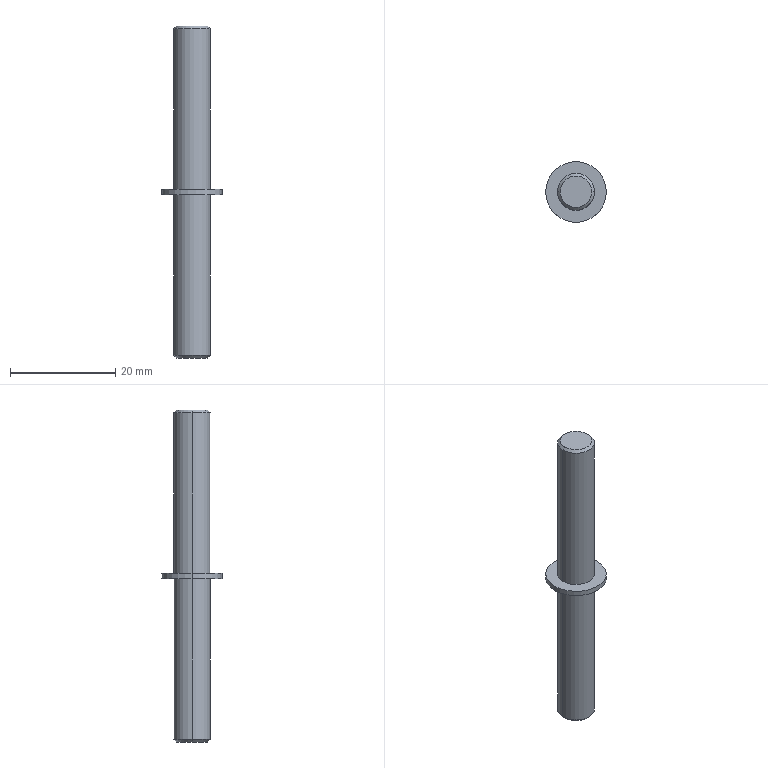Part | NX | features BREP 1 | 1 solid | 14 faces | box 11.5 x 11.5 x 63 mm | volume 2485 mm3 | cylinder 6 | cone 4 | plane 4 | commonest cylinder face diameters 7 x4 11.5 x2
STEP:
#1=CARTESIAN_POINT('',(-3.5,0.,31.));
#2=VERTEX_POINT('',#1);
#3=CARTESIAN_POINT('',(3.5,0.,31.));
#4=VERTEX_POINT('',#3);
#5=CARTESIAN_POINT('',(0.,0.,31.));
#6=DIRECTION('',(0.,0.,-1.));
#7=DIRECTION('',(1.,0.,0.));
#8=AXIS2_PLACEMENT_3D('',#5,#6,#7);
#9=CIRCLE('',#8,3.5);
#10=EDGE_CURVE('',#2,#4,#9,.T.);
#11=ORIENTED_EDGE('',*,*,#10,.T.);
#12=CARTESIAN_POINT('',(3.5,0.,0.5));
#13=VERTEX_POINT('',#12);
#14=CARTESIAN_POINT('',(3.5,0.,31.5));
#15=DIRECTION('',(0.,0.,-1.));
#16=VECTOR('',#15,1000.);
#17=LINE('',#14,#16);
#18=EDGE_CURVE('',#4,#13,#17,.T.);
#19=ORIENTED_EDGE('',*,*,#18,.T.);
#20=CARTESIAN_POINT('',(-3.5,0.,0.5));
#21=VERTEX_POINT('',#20);
#22=CARTESIAN_POINT('',(0.,0.,0.5));
#23=DIRECTION('',(0.,0.,-1.));
#24=DIRECTION('',(-1.,0.,0.));
#25=AXIS2_PLACEMENT_3D('',#22,#23,#24);
#26=CIRCLE('',#25,3.5);
#27=EDGE_CURVE('',#21,#13,#26,.T.);
#28=ORIENTED_EDGE('',*,*,#27,.F.);
#29=CARTESIAN_POINT('',(-3.5,0.,31.5));
#30=DIRECTION('',(0.,0.,-1.));
#31=VECTOR('',#30,1000.);
#32=LINE('',#29,#31);
#33=EDGE_CURVE('',#2,#21,#32,.T.);
#34=ORIENTED_EDGE('',*,*,#33,.F.);
#35=EDGE_LOOP('',(#11,#19,#28,#34));
#36=FACE_BOUND('',#35,.T.);
#37=CARTESIAN_POINT('',(0.,0.,31.5));
#38=DIRECTION('',(0.,0.,-1.));
#39=DIRECTION('',(-1.,0.,0.));
#40=AXIS2_PLACEMENT_3D('',#37,#38,#39);
#41=CYLINDRICAL_SURFACE('',#40,3.5);
#42=ADVANCED_FACE('',(#36),#41,.T.);
#43=CARTESIAN_POINT('',(3.,0.,31.5));
#44=VERTEX_POINT('',#43);
#45=CARTESIAN_POINT('',(-3.,0.,31.5));
#46=VERTEX_POINT('',#45);
#47=CARTESIAN_POINT('',(0.,0.,31.5));
#48=DIRECTION('',(0.,0.,1.));
#49=DIRECTION('',(1.,0.,0.));
#50=AXIS2_PLACEMENT_3D('',#47,#48,#49);
#51=CIRCLE('',#50,3.);
#52=EDGE_CURVE('',#44,#46,#51,.T.);
#53=ORIENTED_EDGE('',*,*,#52,.F.);
#54=CARTESIAN_POINT('',(3.,0.,31.5));
#55=DIRECTION('',(0.7071,0.,-0.7071));
#56=VECTOR('',#55,1000.);
#57=LINE('',#54,#56);
#58=EDGE_CURVE('',#44,#4,#57,.T.);
#59=ORIENTED_EDGE('',*,*,#58,.T.);
#60=ORIENTED_EDGE('',*,*,#10,.F.);
#61=CARTESIAN_POINT('',(-3.,0.,31.5));
#62=DIRECTION('',(-0.7071,0.,-0.7071));
#63=VECTOR('',#62,1000.);
#64=LINE('',#61,#63);
#65=EDGE_CURVE('',#46,#2,#64,.T.);
#66=ORIENTED_EDGE('',*,*,#65,.F.);
#67=EDGE_LOOP('',(#53,#59,#60,#66));
#68=FACE_BOUND('',#67,.T.);
#69=CARTESIAN_POINT('',(0.,0.,31.5));
#70=DIRECTION('',(0.,0.,-1.));
#71=DIRECTION('',(-1.,0.,0.));
#72=AXIS2_PLACEMENT_3D('',#69,#70,#71);
#73=CONICAL_SURFACE('',#72,3.,0.7854);
#74=ADVANCED_FACE('',(#68),#73,.T.);
#75=CARTESIAN_POINT('',(-5.75,0.,0.5));
#76=VERTEX_POINT('',#75);
#77=CARTESIAN_POINT('',(5.75,0.,0.5));
#78=VERTEX_POINT('',#77);
#79=CARTESIAN_POINT('',(0.,0.,0.5));
#80=DIRECTION('',(0.,0.,-1.));
#81=DIRECTION('',(-1.,0.,0.));
#82=AXIS2_PLACEMENT_3D('',#79,#80,#81);
#83=CIRCLE('',#82,5.75);
#84=EDGE_CURVE('',#76,#78,#83,.T.);
#85=ORIENTED_EDGE('',*,*,#84,.T.);
#86=CARTESIAN_POINT('',(5.75,0.,-0.5));
#87=VERTEX_POINT('',#86);
#88=CARTESIAN_POINT('',(5.75,0.,0.));
#89=DIRECTION('',(0.,0.,-1.));
#90=VECTOR('',#89,1000.);
#91=LINE('',#88,#90);
#92=EDGE_CURVE('',#78,#87,#91,.T.);
#93=ORIENTED_EDGE('',*,*,#92,.T.);
#94=CARTESIAN_POINT('',(-5.75,0.,-0.5));
#95=VERTEX_POINT('',#94);
#96=CARTESIAN_POINT('',(0.,0.,-0.5));
#97=DIRECTION('',(0.,0.,-1.));
#98=DIRECTION('',(-1.,0.,0.));
#99=AXIS2_PLACEMENT_3D('',#96,#97,#98);
#100=CIRCLE('',#99,5.75);
#101=EDGE_CURVE('',#95,#87,#100,.T.);
#102=ORIENTED_EDGE('',*,*,#101,.F.);
#103=CARTESIAN_POINT('',(-5.75,0.,0.));
#104=DIRECTION('',(0.,0.,-1.));
#105=VECTOR('',#104,1000.);
#106=LINE('',#103,#105);
#107=EDGE_CURVE('',#76,#95,#106,.T.);
#108=ORIENTED_EDGE('',*,*,#107,.F.);
#109=EDGE_LOOP('',(#85,#93,#102,#108));
#110=FACE_BOUND('',#109,.T.);
#111=CARTESIAN_POINT('',(0.,0.,0.));
#112=DIRECTION('',(0.,0.,-1.));
#113=DIRECTION('',(-1.,0.,0.));
#114=AXIS2_PLACEMENT_3D('',#111,#112,#113);
#115=CYLINDRICAL_SURFACE('',#114,5.75);
#116=ADVANCED_FACE('',(#110),#115,.T.);
#117=CARTESIAN_POINT('',(-3.,0.,-31.5));
#118=VERTEX_POINT('',#117);
#119=CARTESIAN_POINT('',(3.,0.,-31.5));
#120=VERTEX_POINT('',#119);
#121=CARTESIAN_POINT('',(0.,0.,-31.5));
#122=DIRECTION('',(0.,0.,-1.));
#123=DIRECTION('',(1.,0.,0.));
#124=AXIS2_PLACEMENT_3D('',#121,#122,#123);
#125=CIRCLE('',#124,3.);
#126=EDGE_CURVE('',#118,#120,#125,.T.);
#127=ORIENTED_EDGE('',*,*,#126,.F.);
#128=CARTESIAN_POINT('',(-3.5,0.,-31.));
#129=VERTEX_POINT('',#128);
#130=CARTESIAN_POINT('',(-3.5,0.,-31.));
#131=DIRECTION('',(-0.7071,0.,0.7071));
#132=VECTOR('',#131,1000.);
#133=LINE('',#130,#132);
#134=EDGE_CURVE('',#129,#118,#133,.F.);
#135=ORIENTED_EDGE('',*,*,#134,.F.);
#136=CARTESIAN_POINT('',(3.5,0.,-31.));
#137=VERTEX_POINT('',#136);
#138=CARTESIAN_POINT('',(0.,0.,-31.));
#139=DIRECTION('',(0.,0.,1.));
#140=DIRECTION('',(1.,0.,0.));
#141=AXIS2_PLACEMENT_3D('',#138,#139,#140);
#142=CIRCLE('',#141,3.5);
#143=EDGE_CURVE('',#137,#129,#142,.T.);
#144=ORIENTED_EDGE('',*,*,#143,.F.);
#145=CARTESIAN_POINT('',(3.5,0.,-31.));
#146=DIRECTION('',(0.7071,0.,0.7071));
#147=VECTOR('',#146,1000.);
#148=LINE('',#145,#147);
#149=EDGE_CURVE('',#137,#120,#148,.F.);
#150=ORIENTED_EDGE('',*,*,#149,.T.);
#151=EDGE_LOOP('',(#127,#135,#144,#150));
#152=FACE_BOUND('',#151,.T.);
#153=CARTESIAN_POINT('',(0.,0.,-31.));
#154=DIRECTION('',(0.,0.,1.));
#155=DIRECTION('',(1.,0.,0.));
#156=AXIS2_PLACEMENT_3D('',#153,#154,#155);
#157=CONICAL_SURFACE('',#156,3.5,0.7854);
#158=ADVANCED_FACE('',(#152),#157,.T.);
#159=CARTESIAN_POINT('',(3.5,0.,-0.5));
#160=VERTEX_POINT('',#159);
#161=CARTESIAN_POINT('',(-3.5,0.,-0.5));
#162=VERTEX_POINT('',#161);
#163=CARTESIAN_POINT('',(0.,0.,-0.5));
#164=DIRECTION('',(0.,0.,1.));
#165=DIRECTION('',(1.,0.,0.));
#166=AXIS2_PLACEMENT_3D('',#163,#164,#165);
#167=CIRCLE('',#166,3.5);
#168=EDGE_CURVE('',#160,#162,#167,.T.);
#169=ORIENTED_EDGE('',*,*,#168,.F.);
#170=CARTESIAN_POINT('',(3.5,0.,31.5));
#171=DIRECTION('',(0.,0.,-1.));
#172=VECTOR('',#171,1000.);
#173=LINE('',#170,#172);
#174=EDGE_CURVE('',#160,#137,#173,.T.);
#175=ORIENTED_EDGE('',*,*,#174,.T.);
#176=ORIENTED_EDGE('',*,*,#143,.T.);
#177=CARTESIAN_POINT('',(-3.5,0.,31.5));
#178=DIRECTION('',(0.,0.,-1.));
#179=VECTOR('',#178,1000.);
#180=LINE('',#177,#179);
#181=EDGE_CURVE('',#162,#129,#180,.T.);
#182=ORIENTED_EDGE('',*,*,#181,.F.);
#183=EDGE_LOOP('',(#169,#175,#176,#182));
#184=FACE_BOUND('',#183,.T.);
#185=CARTESIAN_POINT('',(0.,0.,31.5));
#186=DIRECTION('',(0.,0.,-1.));
#187=DIRECTION('',(-1.,0.,0.));
#188=AXIS2_PLACEMENT_3D('',#185,#186,#187);
#189=CYLINDRICAL_SURFACE('',#188,3.5);
#190=ADVANCED_FACE('',(#184),#189,.T.);
#191=ORIENTED_EDGE('',*,*,#174,.F.);
#192=CARTESIAN_POINT('',(0.,0.,-0.5));
#193=DIRECTION('',(0.,0.,1.));
#194=DIRECTION('',(1.,0.,0.));
#195=AXIS2_PLACEMENT_3D('',#192,#193,#194);
#196=CIRCLE('',#195,3.5);
#197=EDGE_CURVE('',#162,#160,#196,.T.);
#198=ORIENTED_EDGE('',*,*,#197,.F.);
#199=ORIENTED_EDGE('',*,*,#181,.T.);
#200=CARTESIAN_POINT('',(0.,0.,-31.));
#201=DIRECTION('',(0.,0.,1.));
#202=DIRECTION('',(1.,0.,0.));
#203=AXIS2_PLACEMENT_3D('',#200,#201,#202);
#204=CIRCLE('',#203,3.5);
#205=EDGE_CURVE('',#129,#137,#204,.T.);
#206=ORIENTED_EDGE('',*,*,#205,.T.);
#207=EDGE_LOOP('',(#191,#198,#199,#206));
#208=FACE_BOUND('',#207,.T.);
#209=CARTESIAN_POINT('',(0.,0.,31.5));
#210=DIRECTION('',(0.,0.,-1.));
#211=DIRECTION('',(-1.,0.,0.));
#212=AXIS2_PLACEMENT_3D('',#209,#210,#211);
#213=CYLINDRICAL_SURFACE('',#212,3.5);
#214=ADVANCED_FACE('',(#208),#213,.T.);
#215=CARTESIAN_POINT('',(0.,0.,-31.5));
#216=DIRECTION('',(0.,0.,-1.));
#217=DIRECTION('',(1.,0.,0.));
#218=AXIS2_PLACEMENT_3D('',#215,#216,#217);
#219=CIRCLE('',#218,3.);
#220=EDGE_CURVE('',#120,#118,#219,.T.);
#221=ORIENTED_EDGE('',*,*,#220,.T.);
#222=ORIENTED_EDGE('',*,*,#126,.T.);
#223=EDGE_LOOP('',(#221,#222));
#224=FACE_BOUND('',#223,.T.);
#225=CARTESIAN_POINT('',(0.,0.,-31.5));
#226=DIRECTION('',(0.,0.,1.));
#227=DIRECTION('',(1.,0.,0.));
#228=AXIS2_PLACEMENT_3D('',#225,#226,#227);
#229=PLANE('',#228);
#230=ADVANCED_FACE('',(#224),#229,.F.);
#231=ORIENTED_EDGE('',*,*,#134,.T.);
#232=ORIENTED_EDGE('',*,*,#220,.F.);
#233=ORIENTED_EDGE('',*,*,#149,.F.);
#234=ORIENTED_EDGE('',*,*,#205,.F.);
#235=EDGE_LOOP('',(#231,#232,#233,#234));
#236=FACE_BOUND('',#235,.T.);
#237=CARTESIAN_POINT('',(0.,0.,-31.));
#238=DIRECTION('',(0.,0.,1.));
#239=DIRECTION('',(1.,0.,0.));
#240=AXIS2_PLACEMENT_3D('',#237,#238,#239);
#241=CONICAL_SURFACE('',#240,3.5,0.7854);
#242=ADVANCED_FACE('',(#236),#241,.T.);
#243=ORIENTED_EDGE('',*,*,#101,.T.);
#244=CARTESIAN_POINT('',(0.,0.,-0.5));
#245=DIRECTION('',(0.,0.,-1.));
#246=DIRECTION('',(-1.,0.,0.));
#247=AXIS2_PLACEMENT_3D('',#244,#245,#246);
#248=CIRCLE('',#247,5.75);
#249=EDGE_CURVE('',#87,#95,#248,.T.);
#250=ORIENTED_EDGE('',*,*,#249,.T.);
#251=EDGE_LOOP('',(#243,#250));
#252=FACE_BOUND('',#251,.T.);
#253=ORIENTED_EDGE('',*,*,#197,.T.);
#254=ORIENTED_EDGE('',*,*,#168,.T.);
#255=EDGE_LOOP('',(#253,#254));
#256=FACE_BOUND('',#255,.T.);
#257=CARTESIAN_POINT('',(0.,0.,-0.5));
#258=DIRECTION('',(0.,0.,1.));
#259=DIRECTION('',(1.,0.,0.));
#260=AXIS2_PLACEMENT_3D('',#257,#258,#259);
#261=PLANE('',#260);
#262=ADVANCED_FACE('',(#252,#256),#261,.F.);
#263=ORIENTED_EDGE('',*,*,#84,.F.);
#264=CARTESIAN_POINT('',(0.,0.,0.5));
#265=DIRECTION('',(0.,0.,-1.));
#266=DIRECTION('',(-1.,0.,0.));
#267=AXIS2_PLACEMENT_3D('',#264,#265,#266);
#268=CIRCLE('',#267,5.75);
#269=EDGE_CURVE('',#78,#76,#268,.T.);
#270=ORIENTED_EDGE('',*,*,#269,.F.);
#271=EDGE_LOOP('',(#263,#270));
#272=FACE_BOUND('',#271,.T.);
#273=ORIENTED_EDGE('',*,*,#27,.T.);
#274=CARTESIAN_POINT('',(0.,0.,0.5));
#275=DIRECTION('',(0.,0.,-1.));
#276=DIRECTION('',(-1.,0.,0.));
#277=AXIS2_PLACEMENT_3D('',#274,#275,#276);
#278=CIRCLE('',#277,3.5);
#279=EDGE_CURVE('',#13,#21,#278,.T.);
#280=ORIENTED_EDGE('',*,*,#279,.T.);
#281=EDGE_LOOP('',(#273,#280));
#282=FACE_BOUND('',#281,.T.);
#283=CARTESIAN_POINT('',(0.,0.,0.5));
#284=DIRECTION('',(0.,0.,-1.));
#285=DIRECTION('',(0.,-1.,0.));
#286=AXIS2_PLACEMENT_3D('',#283,#284,#285);
#287=PLANE('',#286);
#288=ADVANCED_FACE('',(#272,#282),#287,.F.);
#289=ORIENTED_EDGE('',*,*,#92,.F.);
#290=ORIENTED_EDGE('',*,*,#269,.T.);
#291=ORIENTED_EDGE('',*,*,#107,.T.);
#292=ORIENTED_EDGE('',*,*,#249,.F.);
#293=EDGE_LOOP('',(#289,#290,#291,#292));
#294=FACE_BOUND('',#293,.T.);
#295=CARTESIAN_POINT('',(0.,0.,0.));
#296=DIRECTION('',(0.,0.,-1.));
#297=DIRECTION('',(-1.,0.,0.));
#298=AXIS2_PLACEMENT_3D('',#295,#296,#297);
#299=CYLINDRICAL_SURFACE('',#298,5.75);
#300=ADVANCED_FACE('',(#294),#299,.T.);
#301=CARTESIAN_POINT('',(0.,0.,31.5));
#302=DIRECTION('',(0.,0.,1.));
#303=DIRECTION('',(1.,0.,0.));
#304=AXIS2_PLACEMENT_3D('',#301,#302,#303);
#305=CIRCLE('',#304,3.);
#306=EDGE_CURVE('',#46,#44,#305,.T.);
#307=ORIENTED_EDGE('',*,*,#306,.T.);
#308=ORIENTED_EDGE('',*,*,#52,.T.);
#309=EDGE_LOOP('',(#307,#308));
#310=FACE_BOUND('',#309,.T.);
#311=CARTESIAN_POINT('',(0.,0.,31.5));
#312=DIRECTION('',(0.,0.,1.));
#313=DIRECTION('',(1.,0.,0.));
#314=AXIS2_PLACEMENT_3D('',#311,#312,#313);
#315=PLANE('',#314);
#316=ADVANCED_FACE('',(#310),#315,.T.);
#317=ORIENTED_EDGE('',*,*,#58,.F.);
#318=ORIENTED_EDGE('',*,*,#306,.F.);
#319=ORIENTED_EDGE('',*,*,#65,.T.);
#320=CARTESIAN_POINT('',(0.,0.,31.));
#321=DIRECTION('',(0.,0.,-1.));
#322=DIRECTION('',(1.,0.,0.));
#323=AXIS2_PLACEMENT_3D('',#320,#321,#322);
#324=CIRCLE('',#323,3.5);
#325=EDGE_CURVE('',#4,#2,#324,.T.);
#326=ORIENTED_EDGE('',*,*,#325,.F.);
#327=EDGE_LOOP('',(#317,#318,#319,#326));
#328=FACE_BOUND('',#327,.T.);
#329=CARTESIAN_POINT('',(0.,0.,31.5));
#330=DIRECTION('',(0.,0.,-1.));
#331=DIRECTION('',(-1.,0.,0.));
#332=AXIS2_PLACEMENT_3D('',#329,#330,#331);
#333=CONICAL_SURFACE('',#332,3.,0.7854);
#334=ADVANCED_FACE('',(#328),#333,.T.);
#335=ORIENTED_EDGE('',*,*,#18,.F.);
#336=ORIENTED_EDGE('',*,*,#325,.T.);
#337=ORIENTED_EDGE('',*,*,#33,.T.);
#338=ORIENTED_EDGE('',*,*,#279,.F.);
#339=EDGE_LOOP('',(#335,#336,#337,#338));
#340=FACE_BOUND('',#339,.T.);
#341=CARTESIAN_POINT('',(0.,0.,31.5));
#342=DIRECTION('',(0.,0.,-1.));
#343=DIRECTION('',(-1.,0.,0.));
#344=AXIS2_PLACEMENT_3D('',#341,#342,#343);
#345=CYLINDRICAL_SURFACE('',#344,3.5);
#346=ADVANCED_FACE('',(#340),#345,.T.);
#347=CLOSED_SHELL('',(#42,#74,#116,#158,#190,#214,#230,#242,#262,#288,#300,#316,#334,#346));
#348=MANIFOLD_SOLID_BREP('',#347);
#349=(LENGTH_UNIT()NAMED_UNIT(*)SI_UNIT(.MILLI.,.METRE.));
#350=UNCERTAINTY_MEASURE_WITH_UNIT(LENGTH_MEASURE(0.00001),#349,'','');
#351=(NAMED_UNIT(*)PLANE_ANGLE_UNIT()SI_UNIT($,.RADIAN.));
#352=(NAMED_UNIT(*)SI_UNIT($,.STERADIAN.)SOLID_ANGLE_UNIT());
#353=(GEOMETRIC_REPRESENTATION_CONTEXT(3)GLOBAL_UNCERTAINTY_ASSIGNED_CONTEXT((#350))GLOBAL_UNIT_ASSIGNED_CONTEXT((#349,#351,#352))REPRESENTATION_CONTEXT('',''));
#354=ADVANCED_BREP_SHAPE_REPRESENTATION('',(#348),#353);